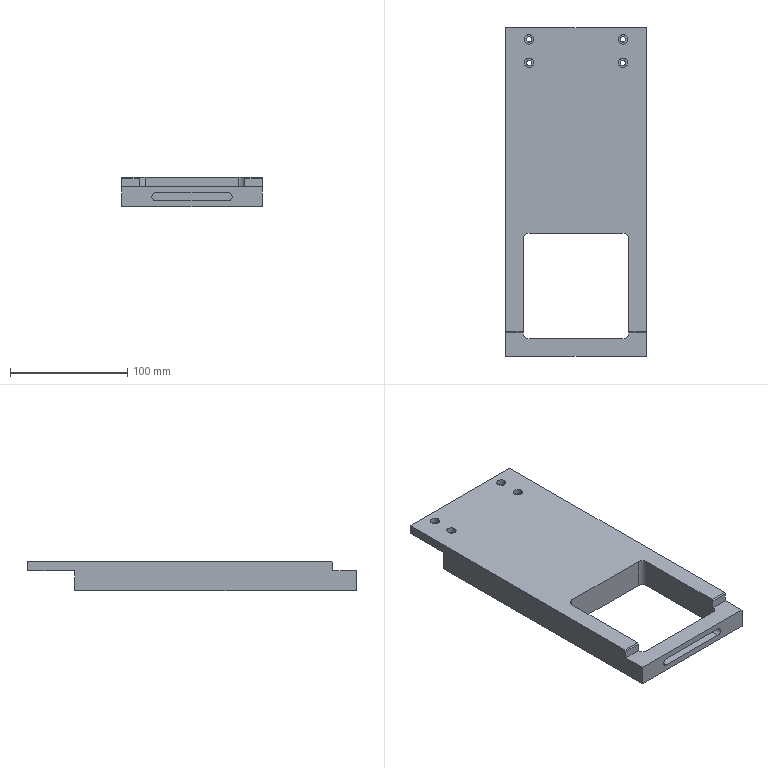Part | STEP file | PN_0020 | 1 solid | 45 faces | box 120 x 280 x 25 mm | volume 533065 mm3 | plane 23 | cylinder 22 | commonest cylinder face diameters 4.5 x8 8 x8 10 x4 6.5 x2